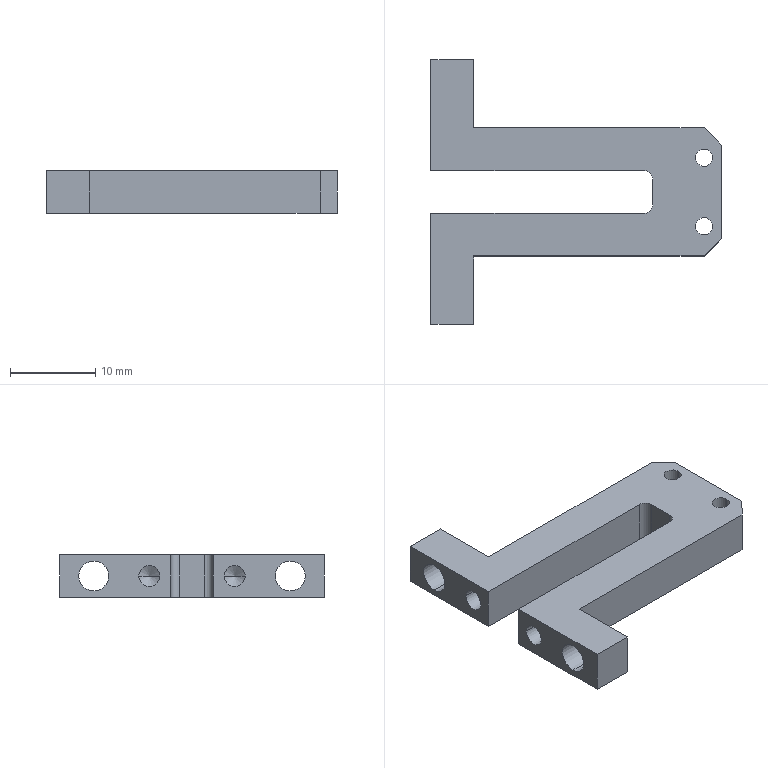Part | SolidWorks | features BaseBody 1 | 1 solid | 34 faces | box 34 x 31 x 5 mm | volume 2038 mm3 | plane 16 | cylinder 14 | cone 4 | commonest cylinder face diameters 2.013 x4 2.459 x4 3.5 x4 2 x2
STEP:
#1=CARTESIAN_POINT('',(5.454,3.851,0.));
#2=VERTEX_POINT('',#1);
#3=CARTESIAN_POINT('',(7.467,3.851,0.));
#4=VERTEX_POINT('',#3);
#5=CARTESIAN_POINT('',(6.461,3.851,0.));
#6=DIRECTION('',(0.,0.,1.));
#7=DIRECTION('',(1.,0.,0.));
#8=AXIS2_PLACEMENT_3D('',#5,#6,#7);
#9=CIRCLE('',#8,1.007);
#10=EDGE_CURVE('',#2,#4,#9,.T.);
#11=ORIENTED_EDGE('',*,*,#10,.F.);
#12=CARTESIAN_POINT('',(5.454,3.851,5.));
#13=VERTEX_POINT('',#12);
#14=CARTESIAN_POINT('',(5.454,3.851,-32.497));
#15=DIRECTION('',(0.,0.,1.));
#16=VECTOR('',#15,1000.);
#17=LINE('',#14,#16);
#18=EDGE_CURVE('',#2,#13,#17,.T.);
#19=ORIENTED_EDGE('',*,*,#18,.T.);
#20=CARTESIAN_POINT('',(7.467,3.851,5.));
#21=VERTEX_POINT('',#20);
#22=CARTESIAN_POINT('',(6.461,3.851,5.));
#23=DIRECTION('',(0.,0.,-1.));
#24=DIRECTION('',(1.,0.,0.));
#25=AXIS2_PLACEMENT_3D('',#22,#23,#24);
#26=CIRCLE('',#25,1.007);
#27=EDGE_CURVE('',#21,#13,#26,.T.);
#28=ORIENTED_EDGE('',*,*,#27,.F.);
#29=CARTESIAN_POINT('',(7.467,3.851,-32.497));
#30=DIRECTION('',(0.,0.,1.));
#31=VECTOR('',#30,1000.);
#32=LINE('',#29,#31);
#33=EDGE_CURVE('',#4,#21,#32,.T.);
#34=ORIENTED_EDGE('',*,*,#33,.F.);
#35=EDGE_LOOP('',(#11,#19,#28,#34));
#36=FACE_OUTER_BOUND('',#35,.T.);
#37=CARTESIAN_POINT('',(6.461,3.851,-32.497));
#38=DIRECTION('',(0.,0.,1.));
#39=DIRECTION('',(1.,0.,0.));
#40=AXIS2_PLACEMENT_3D('',#37,#38,#39);
#41=CYLINDRICAL_SURFACE('',#40,1.007);
#42=ADVANCED_FACE('',(#36),#41,.F.);
#43=CARTESIAN_POINT('',(5.454,-4.149,0.));
#44=VERTEX_POINT('',#43);
#45=CARTESIAN_POINT('',(7.467,-4.149,0.));
#46=VERTEX_POINT('',#45);
#47=CARTESIAN_POINT('',(6.461,-4.149,0.));
#48=DIRECTION('',(0.,0.,1.));
#49=DIRECTION('',(1.,0.,0.));
#50=AXIS2_PLACEMENT_3D('',#47,#48,#49);
#51=CIRCLE('',#50,1.007);
#52=EDGE_CURVE('',#44,#46,#51,.T.);
#53=ORIENTED_EDGE('',*,*,#52,.F.);
#54=CARTESIAN_POINT('',(5.454,-4.149,5.));
#55=VERTEX_POINT('',#54);
#56=CARTESIAN_POINT('',(5.454,-4.149,-32.497));
#57=DIRECTION('',(0.,0.,1.));
#58=VECTOR('',#57,1000.);
#59=LINE('',#56,#58);
#60=EDGE_CURVE('',#44,#55,#59,.T.);
#61=ORIENTED_EDGE('',*,*,#60,.T.);
#62=CARTESIAN_POINT('',(7.467,-4.149,5.));
#63=VERTEX_POINT('',#62);
#64=CARTESIAN_POINT('',(6.461,-4.149,5.));
#65=DIRECTION('',(0.,0.,-1.));
#66=DIRECTION('',(1.,0.,0.));
#67=AXIS2_PLACEMENT_3D('',#64,#65,#66);
#68=CIRCLE('',#67,1.007);
#69=EDGE_CURVE('',#63,#55,#68,.T.);
#70=ORIENTED_EDGE('',*,*,#69,.F.);
#71=CARTESIAN_POINT('',(7.467,-4.149,-32.497));
#72=DIRECTION('',(0.,0.,1.));
#73=VECTOR('',#72,1000.);
#74=LINE('',#71,#73);
#75=EDGE_CURVE('',#46,#63,#74,.T.);
#76=ORIENTED_EDGE('',*,*,#75,.F.);
#77=EDGE_LOOP('',(#53,#61,#70,#76));
#78=FACE_OUTER_BOUND('',#77,.T.);
#79=CARTESIAN_POINT('',(6.461,-4.149,-32.497));
#80=DIRECTION('',(0.,0.,1.));
#81=DIRECTION('',(1.,0.,0.));
#82=AXIS2_PLACEMENT_3D('',#79,#80,#81);
#83=CYLINDRICAL_SURFACE('',#82,1.007);
#84=ADVANCED_FACE('',(#78),#83,.F.);
#85=CARTESIAN_POINT('',(-13.539,6.081,2.5));
#86=VERTEX_POINT('',#85);
#87=CARTESIAN_POINT('',(-13.539,3.622,2.5));
#88=VERTEX_POINT('',#87);
#89=CARTESIAN_POINT('',(-13.539,4.851,2.5));
#90=DIRECTION('',(-1.,0.,0.));
#91=DIRECTION('',(0.,-1.,0.));
#92=AXIS2_PLACEMENT_3D('',#89,#90,#91);
#93=CIRCLE('',#92,1.23);
#94=EDGE_CURVE('',#86,#88,#93,.T.);
#95=ORIENTED_EDGE('',*,*,#94,.F.);
#96=CARTESIAN_POINT('',(-25.539,6.081,2.5));
#97=VERTEX_POINT('',#96);
#98=CARTESIAN_POINT('',(-19.539,6.081,2.5));
#99=DIRECTION('',(-1.,0.,0.));
#100=VECTOR('',#99,1000.);
#101=LINE('',#98,#100);
#102=EDGE_CURVE('',#86,#97,#101,.T.);
#103=ORIENTED_EDGE('',*,*,#102,.T.);
#104=CARTESIAN_POINT('',(-25.539,3.622,2.5));
#105=VERTEX_POINT('',#104);
#106=CARTESIAN_POINT('',(-25.539,4.851,2.5));
#107=DIRECTION('',(1.,0.,0.));
#108=DIRECTION('',(0.,-1.,0.));
#109=AXIS2_PLACEMENT_3D('',#106,#107,#108);
#110=CIRCLE('',#109,1.23);
#111=EDGE_CURVE('',#105,#97,#110,.T.);
#112=ORIENTED_EDGE('',*,*,#111,.F.);
#113=CARTESIAN_POINT('',(-19.539,3.622,2.5));
#114=DIRECTION('',(-1.,0.,0.));
#115=VECTOR('',#114,1000.);
#116=LINE('',#113,#115);
#117=EDGE_CURVE('',#88,#105,#116,.T.);
#118=ORIENTED_EDGE('',*,*,#117,.F.);
#119=EDGE_LOOP('',(#95,#103,#112,#118));
#120=FACE_OUTER_BOUND('',#119,.T.);
#121=CARTESIAN_POINT('',(-19.539,4.851,2.5));
#122=DIRECTION('',(-1.,0.,0.));
#123=DIRECTION('',(0.,-1.,0.));
#124=AXIS2_PLACEMENT_3D('',#121,#122,#123);
#125=CYLINDRICAL_SURFACE('',#124,1.23);
#126=ADVANCED_FACE('',(#120),#125,.F.);
#127=CARTESIAN_POINT('',(-25.539,11.351,4.25));
#128=VERTEX_POINT('',#127);
#129=CARTESIAN_POINT('',(-25.539,11.351,0.75));
#130=VERTEX_POINT('',#129);
#131=CARTESIAN_POINT('',(-25.539,11.351,2.5));
#132=DIRECTION('',(1.,0.,0.));
#133=DIRECTION('',(0.,0.,-1.));
#134=AXIS2_PLACEMENT_3D('',#131,#132,#133);
#135=CIRCLE('',#134,1.75);
#136=EDGE_CURVE('',#128,#130,#135,.T.);
#137=ORIENTED_EDGE('',*,*,#136,.F.);
#138=CARTESIAN_POINT('',(-20.539,11.351,4.25));
#139=VERTEX_POINT('',#138);
#140=CARTESIAN_POINT('',(-66.821,11.351,4.25));
#141=DIRECTION('',(1.,0.,0.));
#142=VECTOR('',#141,1000.);
#143=LINE('',#140,#142);
#144=EDGE_CURVE('',#128,#139,#143,.T.);
#145=ORIENTED_EDGE('',*,*,#144,.T.);
#146=CARTESIAN_POINT('',(-20.539,11.351,0.75));
#147=VERTEX_POINT('',#146);
#148=CARTESIAN_POINT('',(-20.539,11.351,2.5));
#149=DIRECTION('',(-1.,0.,0.));
#150=DIRECTION('',(0.,0.,-1.));
#151=AXIS2_PLACEMENT_3D('',#148,#149,#150);
#152=CIRCLE('',#151,1.75);
#153=EDGE_CURVE('',#147,#139,#152,.T.);
#154=ORIENTED_EDGE('',*,*,#153,.F.);
#155=CARTESIAN_POINT('',(-66.821,11.351,0.75));
#156=DIRECTION('',(1.,0.,0.));
#157=VECTOR('',#156,1000.);
#158=LINE('',#155,#157);
#159=EDGE_CURVE('',#130,#147,#158,.T.);
#160=ORIENTED_EDGE('',*,*,#159,.F.);
#161=EDGE_LOOP('',(#137,#145,#154,#160));
#162=FACE_OUTER_BOUND('',#161,.T.);
#163=CARTESIAN_POINT('',(-66.821,11.351,2.5));
#164=DIRECTION('',(1.,0.,0.));
#165=DIRECTION('',(0.,0.,-1.));
#166=AXIS2_PLACEMENT_3D('',#163,#164,#165);
#167=CYLINDRICAL_SURFACE('',#166,1.75);
#168=ADVANCED_FACE('',(#162),#167,.F.);
#169=CARTESIAN_POINT('',(-25.539,-11.649,4.25));
#170=VERTEX_POINT('',#169);
#171=CARTESIAN_POINT('',(-25.539,-11.649,0.75));
#172=VERTEX_POINT('',#171);
#173=CARTESIAN_POINT('',(-25.539,-11.649,2.5));
#174=DIRECTION('',(1.,0.,0.));
#175=DIRECTION('',(0.,0.,-1.));
#176=AXIS2_PLACEMENT_3D('',#173,#174,#175);
#177=CIRCLE('',#176,1.75);
#178=EDGE_CURVE('',#170,#172,#177,.T.);
#179=ORIENTED_EDGE('',*,*,#178,.F.);
#180=CARTESIAN_POINT('',(-20.539,-11.649,4.25));
#181=VERTEX_POINT('',#180);
#182=CARTESIAN_POINT('',(-66.821,-11.649,4.25));
#183=DIRECTION('',(1.,0.,0.));
#184=VECTOR('',#183,1000.);
#185=LINE('',#182,#184);
#186=EDGE_CURVE('',#170,#181,#185,.T.);
#187=ORIENTED_EDGE('',*,*,#186,.T.);
#188=CARTESIAN_POINT('',(-20.539,-11.649,0.75));
#189=VERTEX_POINT('',#188);
#190=CARTESIAN_POINT('',(-20.539,-11.649,2.5));
#191=DIRECTION('',(-1.,0.,0.));
#192=DIRECTION('',(0.,0.,-1.));
#193=AXIS2_PLACEMENT_3D('',#190,#191,#192);
#194=CIRCLE('',#193,1.75);
#195=EDGE_CURVE('',#189,#181,#194,.T.);
#196=ORIENTED_EDGE('',*,*,#195,.F.);
#197=CARTESIAN_POINT('',(-66.821,-11.649,0.75));
#198=DIRECTION('',(1.,0.,0.));
#199=VECTOR('',#198,1000.);
#200=LINE('',#197,#199);
#201=EDGE_CURVE('',#172,#189,#200,.T.);
#202=ORIENTED_EDGE('',*,*,#201,.F.);
#203=EDGE_LOOP('',(#179,#187,#196,#202));
#204=FACE_OUTER_BOUND('',#203,.T.);
#205=CARTESIAN_POINT('',(-66.821,-11.649,2.5));
#206=DIRECTION('',(1.,0.,0.));
#207=DIRECTION('',(0.,0.,-1.));
#208=AXIS2_PLACEMENT_3D('',#205,#206,#207);
#209=CYLINDRICAL_SURFACE('',#208,1.75);
#210=ADVANCED_FACE('',(#204),#209,.F.);
#211=CARTESIAN_POINT('',(-13.539,-3.919,2.5));
#212=VERTEX_POINT('',#211);
#213=CARTESIAN_POINT('',(-13.539,-6.378,2.5));
#214=VERTEX_POINT('',#213);
#215=CARTESIAN_POINT('',(-13.539,-5.149,2.5));
#216=DIRECTION('',(-1.,0.,0.));
#217=DIRECTION('',(0.,-1.,0.));
#218=AXIS2_PLACEMENT_3D('',#215,#216,#217);
#219=CIRCLE('',#218,1.23);
#220=EDGE_CURVE('',#212,#214,#219,.T.);
#221=ORIENTED_EDGE('',*,*,#220,.F.);
#222=CARTESIAN_POINT('',(-25.539,-3.919,2.5));
#223=VERTEX_POINT('',#222);
#224=CARTESIAN_POINT('',(-19.539,-3.919,2.5));
#225=DIRECTION('',(-1.,0.,0.));
#226=VECTOR('',#225,1000.);
#227=LINE('',#224,#226);
#228=EDGE_CURVE('',#212,#223,#227,.T.);
#229=ORIENTED_EDGE('',*,*,#228,.T.);
#230=CARTESIAN_POINT('',(-25.539,-6.378,2.5));
#231=VERTEX_POINT('',#230);
#232=CARTESIAN_POINT('',(-25.539,-5.149,2.5));
#233=DIRECTION('',(1.,0.,0.));
#234=DIRECTION('',(0.,-1.,0.));
#235=AXIS2_PLACEMENT_3D('',#232,#233,#234);
#236=CIRCLE('',#235,1.23);
#237=EDGE_CURVE('',#231,#223,#236,.T.);
#238=ORIENTED_EDGE('',*,*,#237,.F.);
#239=CARTESIAN_POINT('',(-19.539,-6.378,2.5));
#240=DIRECTION('',(-1.,0.,0.));
#241=VECTOR('',#240,1000.);
#242=LINE('',#239,#241);
#243=EDGE_CURVE('',#214,#231,#242,.T.);
#244=ORIENTED_EDGE('',*,*,#243,.F.);
#245=EDGE_LOOP('',(#221,#229,#238,#244));
#246=FACE_OUTER_BOUND('',#245,.T.);
#247=CARTESIAN_POINT('',(-19.539,-5.149,2.5));
#248=DIRECTION('',(-1.,0.,0.));
#249=DIRECTION('',(0.,-1.,0.));
#250=AXIS2_PLACEMENT_3D('',#247,#248,#249);
#251=CYLINDRICAL_SURFACE('',#250,1.23);
#252=ADVANCED_FACE('',(#246),#251,.F.);
#253=CARTESIAN_POINT('',(-12.8,4.851,2.5));
#254=VERTEX_POINT('',#253);
#255=CARTESIAN_POINT('',(-13.539,3.622,2.5));
#256=DIRECTION('',(-0.515,-0.8572,0.));
#257=VECTOR('',#256,1000.);
#258=LINE('',#255,#257);
#259=EDGE_CURVE('',#254,#88,#258,.T.);
#260=ORIENTED_EDGE('',*,*,#259,.F.);
#261=CARTESIAN_POINT('',(-13.539,6.081,2.5));
#262=DIRECTION('',(-0.515,0.8572,0.));
#263=VECTOR('',#262,1000.);
#264=LINE('',#261,#263);
#265=EDGE_CURVE('',#254,#86,#264,.T.);
#266=ORIENTED_EDGE('',*,*,#265,.T.);
#267=ORIENTED_EDGE('',*,*,#94,.T.);
#268=EDGE_LOOP('',(#260,#266,#267));
#269=FACE_OUTER_BOUND('',#268,.T.);
#270=CARTESIAN_POINT('',(-13.539,4.851,2.5));
#271=DIRECTION('',(-1.,0.,0.));
#272=DIRECTION('',(0.,-1.,0.));
#273=AXIS2_PLACEMENT_3D('',#270,#271,#272);
#274=CONICAL_SURFACE('',#273,1.229,1.03);
#275=ADVANCED_FACE('',(#269),#274,.F.);
#276=CARTESIAN_POINT('',(-12.8,-5.149,2.5));
#277=VERTEX_POINT('',#276);
#278=CARTESIAN_POINT('',(-13.539,-6.378,2.5));
#279=DIRECTION('',(-0.515,-0.8572,0.));
#280=VECTOR('',#279,1000.);
#281=LINE('',#278,#280);
#282=EDGE_CURVE('',#277,#214,#281,.T.);
#283=ORIENTED_EDGE('',*,*,#282,.F.);
#284=CARTESIAN_POINT('',(-13.539,-3.919,2.5));
#285=DIRECTION('',(-0.515,0.8572,0.));
#286=VECTOR('',#285,1000.);
#287=LINE('',#284,#286);
#288=EDGE_CURVE('',#277,#212,#287,.T.);
#289=ORIENTED_EDGE('',*,*,#288,.T.);
#290=ORIENTED_EDGE('',*,*,#220,.T.);
#291=EDGE_LOOP('',(#283,#289,#290));
#292=FACE_OUTER_BOUND('',#291,.T.);
#293=CARTESIAN_POINT('',(-13.539,-5.149,2.5));
#294=DIRECTION('',(-1.,0.,0.));
#295=DIRECTION('',(0.,-1.,0.));
#296=AXIS2_PLACEMENT_3D('',#293,#294,#295);
#297=CONICAL_SURFACE('',#296,1.229,1.03);
#298=ADVANCED_FACE('',(#292),#297,.F.);
#299=ORIENTED_EDGE('',*,*,#27,.T.);
#300=CARTESIAN_POINT('',(6.461,3.851,5.));
#301=DIRECTION('',(0.,0.,-1.));
#302=DIRECTION('',(1.,0.,0.));
#303=AXIS2_PLACEMENT_3D('',#300,#301,#302);
#304=CIRCLE('',#303,1.007);
#305=EDGE_CURVE('',#13,#21,#304,.T.);
#306=ORIENTED_EDGE('',*,*,#305,.T.);
#307=EDGE_LOOP('',(#299,#306));
#308=FACE_BOUND('',#307,.T.);
#309=ORIENTED_EDGE('',*,*,#69,.T.);
#310=CARTESIAN_POINT('',(6.461,-4.149,5.));
#311=DIRECTION('',(0.,0.,-1.));
#312=DIRECTION('',(1.,0.,0.));
#313=AXIS2_PLACEMENT_3D('',#310,#311,#312);
#314=CIRCLE('',#313,1.007);
#315=EDGE_CURVE('',#55,#63,#314,.T.);
#316=ORIENTED_EDGE('',*,*,#315,.T.);
#317=EDGE_LOOP('',(#309,#316));
#318=FACE_BOUND('',#317,.T.);
#319=CARTESIAN_POINT('',(-20.539,15.351,5.));
#320=VERTEX_POINT('',#319);
#321=CARTESIAN_POINT('',(-25.539,15.351,5.));
#322=VERTEX_POINT('',#321);
#323=CARTESIAN_POINT('',(-8.539,15.351,5.));
#324=DIRECTION('',(-1.,0.,0.));
#325=VECTOR('',#324,1000.);
#326=LINE('',#323,#325);
#327=EDGE_CURVE('',#320,#322,#326,.T.);
#328=ORIENTED_EDGE('',*,*,#327,.T.);
#329=CARTESIAN_POINT('',(-25.539,2.351,5.));
#330=VERTEX_POINT('',#329);
#331=CARTESIAN_POINT('',(-25.539,-0.1489,5.));
#332=DIRECTION('',(0.,-1.,0.));
#333=VECTOR('',#332,1000.);
#334=LINE('',#331,#333);
#335=EDGE_CURVE('',#322,#330,#334,.T.);
#336=ORIENTED_EDGE('',*,*,#335,.T.);
#337=CARTESIAN_POINT('',(-0.5392,2.351,5.));
#338=VERTEX_POINT('',#337);
#339=CARTESIAN_POINT('',(-8.539,2.351,5.));
#340=DIRECTION('',(1.,0.,0.));
#341=VECTOR('',#340,1000.);
#342=LINE('',#339,#341);
#343=EDGE_CURVE('',#330,#338,#342,.T.);
#344=ORIENTED_EDGE('',*,*,#343,.T.);
#345=CARTESIAN_POINT('',(0.4608,1.351,5.));
#346=VERTEX_POINT('',#345);
#347=CARTESIAN_POINT('',(-0.5392,1.351,5.));
#348=DIRECTION('',(0.,0.,-1.));
#349=DIRECTION('',(-1.,0.,0.));
#350=AXIS2_PLACEMENT_3D('',#347,#348,#349);
#351=CIRCLE('',#350,1.);
#352=EDGE_CURVE('',#338,#346,#351,.T.);
#353=ORIENTED_EDGE('',*,*,#352,.T.);
#354=CARTESIAN_POINT('',(0.4608,-1.649,5.));
#355=VERTEX_POINT('',#354);
#356=CARTESIAN_POINT('',(0.4608,-0.1489,5.));
#357=DIRECTION('',(0.,-1.,0.));
#358=VECTOR('',#357,1000.);
#359=LINE('',#356,#358);
#360=EDGE_CURVE('',#346,#355,#359,.T.);
#361=ORIENTED_EDGE('',*,*,#360,.T.);
#362=CARTESIAN_POINT('',(-0.5392,-2.649,5.));
#363=VERTEX_POINT('',#362);
#364=CARTESIAN_POINT('',(-0.5392,-1.649,5.));
#365=DIRECTION('',(0.,0.,-1.));
#366=DIRECTION('',(-1.,0.,0.));
#367=AXIS2_PLACEMENT_3D('',#364,#365,#366);
#368=CIRCLE('',#367,1.);
#369=EDGE_CURVE('',#355,#363,#368,.T.);
#370=ORIENTED_EDGE('',*,*,#369,.T.);
#371=CARTESIAN_POINT('',(-25.539,-2.649,5.));
#372=VERTEX_POINT('',#371);
#373=CARTESIAN_POINT('',(-8.539,-2.649,5.));
#374=DIRECTION('',(-1.,0.,0.));
#375=VECTOR('',#374,1000.);
#376=LINE('',#373,#375);
#377=EDGE_CURVE('',#363,#372,#376,.T.);
#378=ORIENTED_EDGE('',*,*,#377,.T.);
#379=CARTESIAN_POINT('',(-25.539,-15.649,5.));
#380=VERTEX_POINT('',#379);
#381=CARTESIAN_POINT('',(-25.539,-0.1489,5.));
#382=DIRECTION('',(0.,-1.,0.));
#383=VECTOR('',#382,1000.);
#384=LINE('',#381,#383);
#385=EDGE_CURVE('',#372,#380,#384,.T.);
#386=ORIENTED_EDGE('',*,*,#385,.T.);
#387=CARTESIAN_POINT('',(-20.539,-15.649,5.));
#388=VERTEX_POINT('',#387);
#389=CARTESIAN_POINT('',(-8.539,-15.649,5.));
#390=DIRECTION('',(1.,0.,0.));
#391=VECTOR('',#390,1000.);
#392=LINE('',#389,#391);
#393=EDGE_CURVE('',#380,#388,#392,.T.);
#394=ORIENTED_EDGE('',*,*,#393,.T.);
#395=CARTESIAN_POINT('',(-20.539,-7.649,5.));
#396=VERTEX_POINT('',#395);
#397=CARTESIAN_POINT('',(-20.539,-0.1489,5.));
#398=DIRECTION('',(0.,1.,0.));
#399=VECTOR('',#398,1000.);
#400=LINE('',#397,#399);
#401=EDGE_CURVE('',#388,#396,#400,.T.);
#402=ORIENTED_EDGE('',*,*,#401,.T.);
#403=CARTESIAN_POINT('',(6.461,-7.649,5.));
#404=VERTEX_POINT('',#403);
#405=CARTESIAN_POINT('',(-8.539,-7.649,5.));
#406=DIRECTION('',(1.,0.,0.));
#407=VECTOR('',#406,1000.);
#408=LINE('',#405,#407);
#409=EDGE_CURVE('',#396,#404,#408,.T.);
#410=ORIENTED_EDGE('',*,*,#409,.T.);
#411=CARTESIAN_POINT('',(8.461,-5.649,5.));
#412=VERTEX_POINT('',#411);
#413=CARTESIAN_POINT('',(6.461,-7.649,5.));
#414=DIRECTION('',(0.7071,0.7071,0.));
#415=VECTOR('',#414,1000.);
#416=LINE('',#413,#415);
#417=EDGE_CURVE('',#404,#412,#416,.T.);
#418=ORIENTED_EDGE('',*,*,#417,.T.);
#419=CARTESIAN_POINT('',(8.461,5.351,5.));
#420=VERTEX_POINT('',#419);
#421=CARTESIAN_POINT('',(8.461,-0.1489,5.));
#422=DIRECTION('',(0.,1.,0.));
#423=VECTOR('',#422,1000.);
#424=LINE('',#421,#423);
#425=EDGE_CURVE('',#412,#420,#424,.T.);
#426=ORIENTED_EDGE('',*,*,#425,.T.);
#427=CARTESIAN_POINT('',(6.461,7.351,5.));
#428=VERTEX_POINT('',#427);
#429=CARTESIAN_POINT('',(8.461,5.351,5.));
#430=DIRECTION('',(-0.7071,0.7071,0.));
#431=VECTOR('',#430,1000.);
#432=LINE('',#429,#431);
#433=EDGE_CURVE('',#420,#428,#432,.T.);
#434=ORIENTED_EDGE('',*,*,#433,.T.);
#435=CARTESIAN_POINT('',(-20.539,7.351,5.));
#436=VERTEX_POINT('',#435);
#437=CARTESIAN_POINT('',(-8.539,7.351,5.));
#438=DIRECTION('',(-1.,0.,0.));
#439=VECTOR('',#438,1000.);
#440=LINE('',#437,#439);
#441=EDGE_CURVE('',#428,#436,#440,.T.);
#442=ORIENTED_EDGE('',*,*,#441,.T.);
#443=CARTESIAN_POINT('',(-20.539,-0.1489,5.));
#444=DIRECTION('',(0.,1.,0.));
#445=VECTOR('',#444,1000.);
#446=LINE('',#443,#445);
#447=EDGE_CURVE('',#436,#320,#446,.T.);
#448=ORIENTED_EDGE('',*,*,#447,.T.);
#449=EDGE_LOOP('',(#328,#336,#344,#353,#361,#370,#378,#386,#394,#402,#410,#418,#426,#434,#442,#448));
#450=FACE_OUTER_BOUND('',#449,.T.);
#451=CARTESIAN_POINT('',(-8.539,-0.1489,5.));
#452=DIRECTION('',(0.,0.,1.));
#453=DIRECTION('',(1.,0.,0.));
#454=AXIS2_PLACEMENT_3D('',#451,#452,#453);
#455=PLANE('',#454);
#456=ADVANCED_FACE('',(#308,#318,#450),#455,.T.);
#457=ORIENTED_EDGE('',*,*,#18,.F.);
#458=CARTESIAN_POINT('',(6.461,3.851,0.));
#459=DIRECTION('',(0.,0.,1.));
#460=DIRECTION('',(1.,0.,0.));
#461=AXIS2_PLACEMENT_3D('',#458,#459,#460);
#462=CIRCLE('',#461,1.007);
#463=EDGE_CURVE('',#4,#2,#462,.T.);
#464=ORIENTED_EDGE('',*,*,#463,.F.);
#465=ORIENTED_EDGE('',*,*,#33,.T.);
#466=ORIENTED_EDGE('',*,*,#305,.F.);
#467=EDGE_LOOP('',(#457,#464,#465,#466));
#468=FACE_OUTER_BOUND('',#467,.T.);
#469=CARTESIAN_POINT('',(6.461,3.851,-32.497));
#470=DIRECTION('',(0.,0.,1.));
#471=DIRECTION('',(1.,0.,0.));
#472=AXIS2_PLACEMENT_3D('',#469,#470,#471);
#473=CYLINDRICAL_SURFACE('',#472,1.007);
#474=ADVANCED_FACE('',(#468),#473,.F.);
#475=ORIENTED_EDGE('',*,*,#60,.F.);
#476=CARTESIAN_POINT('',(6.461,-4.149,0.));
#477=DIRECTION('',(0.,0.,1.));
#478=DIRECTION('',(1.,0.,0.));
#479=AXIS2_PLACEMENT_3D('',#476,#477,#478);
#480=CIRCLE('',#479,1.007);
#481=EDGE_CURVE('',#46,#44,#480,.T.);
#482=ORIENTED_EDGE('',*,*,#481,.F.);
#483=ORIENTED_EDGE('',*,*,#75,.T.);
#484=ORIENTED_EDGE('',*,*,#315,.F.);
#485=EDGE_LOOP('',(#475,#482,#483,#484));
#486=FACE_OUTER_BOUND('',#485,.T.);
#487=CARTESIAN_POINT('',(6.461,-4.149,-32.497));
#488=DIRECTION('',(0.,0.,1.));
#489=DIRECTION('',(1.,0.,0.));
#490=AXIS2_PLACEMENT_3D('',#487,#488,#489);
#491=CYLINDRICAL_SURFACE('',#490,1.007);
#492=ADVANCED_FACE('',(#486),#491,.F.);
#493=ORIENTED_EDGE('',*,*,#111,.T.);
#494=CARTESIAN_POINT('',(-25.539,4.851,2.5));
#495=DIRECTION('',(1.,0.,0.));
#496=DIRECTION('',(0.,-1.,0.));
#497=AXIS2_PLACEMENT_3D('',#494,#495,#496);
#498=CIRCLE('',#497,1.23);
#499=EDGE_CURVE('',#97,#105,#498,.T.);
#500=ORIENTED_EDGE('',*,*,#499,.T.);
#501=EDGE_LOOP('',(#493,#500));
#502=FACE_BOUND('',#501,.T.);
#503=CARTESIAN_POINT('',(-25.539,11.351,2.5));
#504=DIRECTION('',(1.,0.,0.));
#505=DIRECTION('',(0.,0.,-1.));
#506=AXIS2_PLACEMENT_3D('',#503,#504,#505);
#507=CIRCLE('',#506,1.75);
#508=EDGE_CURVE('',#130,#128,#507,.T.);
#509=ORIENTED_EDGE('',*,*,#508,.T.);
#510=ORIENTED_EDGE('',*,*,#136,.T.);
#511=EDGE_LOOP('',(#509,#510));
#512=FACE_BOUND('',#511,.T.);
#513=CARTESIAN_POINT('',(-25.539,15.351,0.));
#514=VERTEX_POINT('',#513);
#515=CARTESIAN_POINT('',(-25.539,15.351,0.));
#516=DIRECTION('',(0.,0.,-1.));
#517=VECTOR('',#516,1000.);
#518=LINE('',#515,#517);
#519=EDGE_CURVE('',#322,#514,#518,.T.);
#520=ORIENTED_EDGE('',*,*,#519,.T.);
#521=CARTESIAN_POINT('',(-25.539,2.351,0.));
#522=VERTEX_POINT('',#521);
#523=CARTESIAN_POINT('',(-25.539,-7.649,0.));
#524=DIRECTION('',(0.,-1.,0.));
#525=VECTOR('',#524,1000.);
#526=LINE('',#523,#525);
#527=EDGE_CURVE('',#514,#522,#526,.T.);
#528=ORIENTED_EDGE('',*,*,#527,.T.);
#529=CARTESIAN_POINT('',(-25.539,2.351,0.));
#530=DIRECTION('',(0.,0.,1.));
#531=VECTOR('',#530,1000.);
#532=LINE('',#529,#531);
#533=EDGE_CURVE('',#522,#330,#532,.T.);
#534=ORIENTED_EDGE('',*,*,#533,.T.);
#535=ORIENTED_EDGE('',*,*,#335,.F.);
#536=EDGE_LOOP('',(#520,#528,#534,#535));
#537=FACE_OUTER_BOUND('',#536,.T.);
#538=CARTESIAN_POINT('',(-25.539,-7.649,0.));
#539=DIRECTION('',(-1.,0.,0.));
#540=DIRECTION('',(0.,0.,1.));
#541=AXIS2_PLACEMENT_3D('',#538,#539,#540);
#542=PLANE('',#541);
#543=ADVANCED_FACE('',(#502,#512,#537),#542,.T.);
#544=ORIENTED_EDGE('',*,*,#327,.F.);
#545=CARTESIAN_POINT('',(-20.539,15.351,0.));
#546=VERTEX_POINT('',#545);
#547=CARTESIAN_POINT('',(-20.539,15.351,2.5));
#548=DIRECTION('',(0.,0.,-1.));
#549=VECTOR('',#548,1000.);
#550=LINE('',#547,#549);
#551=EDGE_CURVE('',#320,#546,#550,.T.);
#552=ORIENTED_EDGE('',*,*,#551,.T.);
#553=CARTESIAN_POINT('',(-23.039,15.351,0.));
#554=DIRECTION('',(-1.,0.,0.));
#555=VECTOR('',#554,1000.);
#556=LINE('',#553,#555);
#557=EDGE_CURVE('',#546,#514,#556,.T.);
#558=ORIENTED_EDGE('',*,*,#557,.T.);
#559=ORIENTED_EDGE('',*,*,#519,.F.);
#560=EDGE_LOOP('',(#544,#552,#558,#559));
#561=FACE_OUTER_BOUND('',#560,.T.);
#562=CARTESIAN_POINT('',(-23.039,15.351,2.5));
#563=DIRECTION('',(0.,1.,0.));
#564=DIRECTION('',(0.,0.,1.));
#565=AXIS2_PLACEMENT_3D('',#562,#563,#564);
#566=PLANE('',#565);
#567=ADVANCED_FACE('',(#561),#566,.T.);
#568=ORIENTED_EDGE('',*,*,#153,.T.);
#569=CARTESIAN_POINT('',(-20.539,11.351,2.5));
#570=DIRECTION('',(-1.,0.,0.));
#571=DIRECTION('',(0.,0.,-1.));
#572=AXIS2_PLACEMENT_3D('',#569,#570,#571);
#573=CIRCLE('',#572,1.75);
#574=EDGE_CURVE('',#139,#147,#573,.T.);
#575=ORIENTED_EDGE('',*,*,#574,.T.);
#576=EDGE_LOOP('',(#568,#575));
#577=FACE_BOUND('',#576,.T.);
#578=CARTESIAN_POINT('',(-20.539,7.351,0.));
#579=VERTEX_POINT('',#578);
#580=CARTESIAN_POINT('',(-20.539,7.351,0.));
#581=DIRECTION('',(0.,0.,-1.));
#582=VECTOR('',#581,1000.);
#583=LINE('',#580,#582);
#584=EDGE_CURVE('',#436,#579,#583,.T.);
#585=ORIENTED_EDGE('',*,*,#584,.T.);
#586=CARTESIAN_POINT('',(-20.539,7.351,0.));
#587=DIRECTION('',(0.,1.,0.));
#588=VECTOR('',#587,1000.);
#589=LINE('',#586,#588);
#590=EDGE_CURVE('',#579,#546,#589,.T.);
#591=ORIENTED_EDGE('',*,*,#590,.T.);
#592=ORIENTED_EDGE('',*,*,#551,.F.);
#593=ORIENTED_EDGE('',*,*,#447,.F.);
#594=EDGE_LOOP('',(#585,#591,#592,#593));
#595=FACE_OUTER_BOUND('',#594,.T.);
#596=CARTESIAN_POINT('',(-20.539,7.351,0.));
#597=DIRECTION('',(1.,0.,0.));
#598=DIRECTION('',(0.,0.,-1.));
#599=AXIS2_PLACEMENT_3D('',#596,#597,#598);
#600=PLANE('',#599);
#601=ADVANCED_FACE('',(#577,#595),#600,.T.);
#602=CARTESIAN_POINT('',(6.461,7.351,0.));
#603=VERTEX_POINT('',#602);
#604=CARTESIAN_POINT('',(6.461,7.351,0.));
#605=DIRECTION('',(0.,0.,-1.));
#606=VECTOR('',#605,1000.);
#607=LINE('',#604,#606);
#608=EDGE_CURVE('',#428,#603,#607,.T.);
#609=ORIENTED_EDGE('',*,*,#608,.T.);
#610=CARTESIAN_POINT('',(-25.539,7.351,0.));
#611=DIRECTION('',(-1.,0.,0.));
#612=VECTOR('',#611,1000.);
#613=LINE('',#610,#612);
#614=EDGE_CURVE('',#603,#579,#613,.T.);
#615=ORIENTED_EDGE('',*,*,#614,.T.);
#616=ORIENTED_EDGE('',*,*,#584,.F.);
#617=ORIENTED_EDGE('',*,*,#441,.F.);
#618=EDGE_LOOP('',(#609,#615,#616,#617));
#619=FACE_OUTER_BOUND('',#618,.T.);
#620=CARTESIAN_POINT('',(-25.539,7.351,0.));
#621=DIRECTION('',(0.,1.,0.));
#622=DIRECTION('',(0.,0.,1.));
#623=AXIS2_PLACEMENT_3D('',#620,#621,#622);
#624=PLANE('',#623);
#625=ADVANCED_FACE('',(#619),#624,.T.);
#626=CARTESIAN_POINT('',(8.461,5.351,0.));
#627=VERTEX_POINT('',#626);
#628=CARTESIAN_POINT('',(7.461,6.351,0.));
#629=DIRECTION('',(-0.7071,0.7071,0.));
#630=VECTOR('',#629,1000.);
#631=LINE('',#628,#630);
#632=EDGE_CURVE('',#627,#603,#631,.T.);
#633=ORIENTED_EDGE('',*,*,#632,.T.);
#634=ORIENTED_EDGE('',*,*,#608,.F.);
#635=ORIENTED_EDGE('',*,*,#433,.F.);
#636=CARTESIAN_POINT('',(8.461,5.351,0.));
#637=DIRECTION('',(0.,0.,-1.));
#638=VECTOR('',#637,1000.);
#639=LINE('',#636,#638);
#640=EDGE_CURVE('',#420,#627,#639,.T.);
#641=ORIENTED_EDGE('',*,*,#640,.T.);
#642=EDGE_LOOP('',(#633,#634,#635,#641));
#643=FACE_OUTER_BOUND('',#642,.T.);
#644=CARTESIAN_POINT('',(7.461,6.351,0.));
#645=DIRECTION('',(0.7071,0.7071,0.));
#646=DIRECTION('',(-0.7071,0.7071,0.));
#647=AXIS2_PLACEMENT_3D('',#644,#645,#646);
#648=PLANE('',#647);
#649=ADVANCED_FACE('',(#643),#648,.T.);
#650=ORIENTED_EDGE('',*,*,#640,.F.);
#651=ORIENTED_EDGE('',*,*,#425,.F.);
#652=CARTESIAN_POINT('',(8.461,-5.649,0.));
#653=VERTEX_POINT('',#652);
#654=CARTESIAN_POINT('',(8.461,-5.649,0.));
#655=DIRECTION('',(0.,0.,-1.));
#656=VECTOR('',#655,1000.);
#657=LINE('',#654,#656);
#658=EDGE_CURVE('',#412,#653,#657,.T.);
#659=ORIENTED_EDGE('',*,*,#658,.T.);
#660=CARTESIAN_POINT('',(8.461,7.351,0.));
#661=DIRECTION('',(0.,1.,0.));
#662=VECTOR('',#661,1000.);
#663=LINE('',#660,#662);
#664=EDGE_CURVE('',#653,#627,#663,.T.);
#665=ORIENTED_EDGE('',*,*,#664,.T.);
#666=EDGE_LOOP('',(#650,#651,#659,#665));
#667=FACE_OUTER_BOUND('',#666,.T.);
#668=CARTESIAN_POINT('',(8.461,7.351,0.));
#669=DIRECTION('',(1.,0.,0.));
#670=DIRECTION('',(0.,0.,-1.));
#671=AXIS2_PLACEMENT_3D('',#668,#669,#670);
#672=PLANE('',#671);
#673=ADVANCED_FACE('',(#667),#672,.T.);
#674=CARTESIAN_POINT('',(6.461,-7.649,0.));
#675=VERTEX_POINT('',#674);
#676=CARTESIAN_POINT('',(7.461,-6.649,0.));
#677=DIRECTION('',(0.7071,0.7071,0.));
#678=VECTOR('',#677,1000.);
#679=LINE('',#676,#678);
#680=EDGE_CURVE('',#675,#653,#679,.T.);
#681=ORIENTED_EDGE('',*,*,#680,.T.);
#682=ORIENTED_EDGE('',*,*,#658,.F.);
#683=ORIENTED_EDGE('',*,*,#417,.F.);
#684=CARTESIAN_POINT('',(6.461,-7.649,0.));
#685=DIRECTION('',(0.,0.,-1.));
#686=VECTOR('',#685,1000.);
#687=LINE('',#684,#686);
#688=EDGE_CURVE('',#404,#675,#687,.T.);
#689=ORIENTED_EDGE('',*,*,#688,.T.);
#690=EDGE_LOOP('',(#681,#682,#683,#689));
#691=FACE_OUTER_BOUND('',#690,.T.);
#692=CARTESIAN_POINT('',(7.461,-6.649,0.));
#693=DIRECTION('',(0.7071,-0.7071,0.));
#694=DIRECTION('',(0.7071,0.7071,0.));
#695=AXIS2_PLACEMENT_3D('',#692,#693,#694);
#696=PLANE('',#695);
#697=ADVANCED_FACE('',(#691),#696,.T.);
#698=ORIENTED_EDGE('',*,*,#688,.F.);
#699=ORIENTED_EDGE('',*,*,#409,.F.);
#700=CARTESIAN_POINT('',(-20.539,-7.649,0.));
#701=VERTEX_POINT('',#700);
#702=CARTESIAN_POINT('',(-20.539,-7.649,0.));
#703=DIRECTION('',(0.,0.,-1.));
#704=VECTOR('',#703,1000.);
#705=LINE('',#702,#704);
#706=EDGE_CURVE('',#396,#701,#705,.T.);
#707=ORIENTED_EDGE('',*,*,#706,.T.);
#708=CARTESIAN_POINT('',(8.461,-7.649,0.));
#709=DIRECTION('',(1.,0.,0.));
#710=VECTOR('',#709,1000.);
#711=LINE('',#708,#710);
#712=EDGE_CURVE('',#701,#675,#711,.T.);
#713=ORIENTED_EDGE('',*,*,#712,.T.);
#714=EDGE_LOOP('',(#698,#699,#707,#713));
#715=FACE_OUTER_BOUND('',#714,.T.);
#716=CARTESIAN_POINT('',(8.461,-7.649,0.));
#717=DIRECTION('',(0.,-1.,0.));
#718=DIRECTION('',(0.,0.,-1.));
#719=AXIS2_PLACEMENT_3D('',#716,#717,#718);
#720=PLANE('',#719);
#721=ADVANCED_FACE('',(#715),#720,.T.);
#722=ORIENTED_EDGE('',*,*,#195,.T.);
#723=CARTESIAN_POINT('',(-20.539,-11.649,2.5));
#724=DIRECTION('',(-1.,0.,0.));
#725=DIRECTION('',(0.,0.,-1.));
#726=AXIS2_PLACEMENT_3D('',#723,#724,#725);
#727=CIRCLE('',#726,1.75);
#728=EDGE_CURVE('',#181,#189,#727,.T.);
#729=ORIENTED_EDGE('',*,*,#728,.T.);
#730=EDGE_LOOP('',(#722,#729));
#731=FACE_BOUND('',#730,.T.);
#732=ORIENTED_EDGE('',*,*,#706,.F.);
#733=ORIENTED_EDGE('',*,*,#401,.F.);
#734=CARTESIAN_POINT('',(-20.539,-15.649,0.));
#735=VERTEX_POINT('',#734);
#736=CARTESIAN_POINT('',(-20.539,-15.649,5.));
#737=DIRECTION('',(0.,0.,-1.));
#738=VECTOR('',#737,1000.);
#739=LINE('',#736,#738);
#740=EDGE_CURVE('',#388,#735,#739,.T.);
#741=ORIENTED_EDGE('',*,*,#740,.T.);
#742=CARTESIAN_POINT('',(-20.539,-7.649,0.));
#743=DIRECTION('',(0.,1.,0.));
#744=VECTOR('',#743,1000.);
#745=LINE('',#742,#744);
#746=EDGE_CURVE('',#735,#701,#745,.T.);
#747=ORIENTED_EDGE('',*,*,#746,.T.);
#748=EDGE_LOOP('',(#732,#733,#741,#747));
#749=FACE_OUTER_BOUND('',#748,.T.);
#750=CARTESIAN_POINT('',(-20.539,-7.649,5.));
#751=DIRECTION('',(1.,0.,0.));
#752=DIRECTION('',(0.,0.,-1.));
#753=AXIS2_PLACEMENT_3D('',#750,#751,#752);
#754=PLANE('',#753);
#755=ADVANCED_FACE('',(#731,#749),#754,.T.);
#756=CARTESIAN_POINT('',(-25.539,-15.649,0.));
#757=VERTEX_POINT('',#756);
#758=CARTESIAN_POINT('',(-25.539,-15.649,2.5));
#759=DIRECTION('',(0.,0.,1.));
#760=VECTOR('',#759,1000.);
#761=LINE('',#758,#760);
#762=EDGE_CURVE('',#757,#380,#761,.T.);
#763=ORIENTED_EDGE('',*,*,#762,.F.);
#764=CARTESIAN_POINT('',(-23.039,-15.649,0.));
#765=DIRECTION('',(-1.,0.,0.));
#766=VECTOR('',#765,1000.);
#767=LINE('',#764,#766);
#768=EDGE_CURVE('',#735,#757,#767,.T.);
#769=ORIENTED_EDGE('',*,*,#768,.F.);
#770=ORIENTED_EDGE('',*,*,#740,.F.);
#771=ORIENTED_EDGE('',*,*,#393,.F.);
#772=EDGE_LOOP('',(#763,#769,#770,#771));
#773=FACE_OUTER_BOUND('',#772,.T.);
#774=CARTESIAN_POINT('',(-23.039,-15.649,2.5));
#775=DIRECTION('',(0.,1.,0.));
#776=DIRECTION('',(0.,0.,1.));
#777=AXIS2_PLACEMENT_3D('',#774,#775,#776);
#778=PLANE('',#777);
#779=ADVANCED_FACE('',(#773),#778,.F.);
#780=ORIENTED_EDGE('',*,*,#237,.T.);
#781=CARTESIAN_POINT('',(-25.539,-5.149,2.5));
#782=DIRECTION('',(1.,0.,0.));
#783=DIRECTION('',(0.,-1.,0.));
#784=AXIS2_PLACEMENT_3D('',#781,#782,#783);
#785=CIRCLE('',#784,1.23);
#786=EDGE_CURVE('',#223,#231,#785,.T.);
#787=ORIENTED_EDGE('',*,*,#786,.T.);
#788=EDGE_LOOP('',(#780,#787));
#789=FACE_BOUND('',#788,.T.);
#790=CARTESIAN_POINT('',(-25.539,-11.649,2.5));
#791=DIRECTION('',(1.,0.,0.));
#792=DIRECTION('',(0.,0.,-1.));
#793=AXIS2_PLACEMENT_3D('',#790,#791,#792);
#794=CIRCLE('',#793,1.75);
#795=EDGE_CURVE('',#172,#170,#794,.T.);
#796=ORIENTED_EDGE('',*,*,#795,.T.);
#797=ORIENTED_EDGE('',*,*,#178,.T.);
#798=EDGE_LOOP('',(#796,#797));
#799=FACE_BOUND('',#798,.T.);
#800=ORIENTED_EDGE('',*,*,#762,.T.);
#801=ORIENTED_EDGE('',*,*,#385,.F.);
#802=CARTESIAN_POINT('',(-25.539,-2.649,0.));
#803=VERTEX_POINT('',#802);
#804=CARTESIAN_POINT('',(-25.539,-2.649,0.));
#805=DIRECTION('',(0.,0.,-1.));
#806=VECTOR('',#805,1000.);
#807=LINE('',#804,#806);
#808=EDGE_CURVE('',#372,#803,#807,.T.);
#809=ORIENTED_EDGE('',*,*,#808,.T.);
#810=CARTESIAN_POINT('',(-25.539,-7.649,0.));
#811=DIRECTION('',(0.,-1.,0.));
#812=VECTOR('',#811,1000.);
#813=LINE('',#810,#812);
#814=EDGE_CURVE('',#803,#757,#813,.T.);
#815=ORIENTED_EDGE('',*,*,#814,.T.);
#816=EDGE_LOOP('',(#800,#801,#809,#815));
#817=FACE_OUTER_BOUND('',#816,.T.);
#818=CARTESIAN_POINT('',(-25.539,-7.649,0.));
#819=DIRECTION('',(-1.,0.,0.));
#820=DIRECTION('',(0.,0.,1.));
#821=AXIS2_PLACEMENT_3D('',#818,#819,#820);
#822=PLANE('',#821);
#823=ADVANCED_FACE('',(#789,#799,#817),#822,.T.);
#824=CARTESIAN_POINT('',(-0.5392,-2.649,0.));
#825=VERTEX_POINT('',#824);
#826=CARTESIAN_POINT('',(-25.539,-2.649,0.));
#827=DIRECTION('',(1.,0.,0.));
#828=VECTOR('',#827,1000.);
#829=LINE('',#826,#828);
#830=EDGE_CURVE('',#803,#825,#829,.T.);
#831=ORIENTED_EDGE('',*,*,#830,.F.);
#832=ORIENTED_EDGE('',*,*,#808,.F.);
#833=ORIENTED_EDGE('',*,*,#377,.F.);
#834=CARTESIAN_POINT('',(-0.5392,-2.649,5.));
#835=DIRECTION('',(0.,0.,1.));
#836=VECTOR('',#835,1000.);
#837=LINE('',#834,#836);
#838=EDGE_CURVE('',#825,#363,#837,.T.);
#839=ORIENTED_EDGE('',*,*,#838,.F.);
#840=EDGE_LOOP('',(#831,#832,#833,#839));
#841=FACE_OUTER_BOUND('',#840,.T.);
#842=CARTESIAN_POINT('',(-25.539,-2.649,5.));
#843=DIRECTION('',(0.,-1.,0.));
#844=DIRECTION('',(0.,0.,-1.));
#845=AXIS2_PLACEMENT_3D('',#842,#843,#844);
#846=PLANE('',#845);
#847=ADVANCED_FACE('',(#841),#846,.F.);
#848=ORIENTED_EDGE('',*,*,#360,.F.);
#849=CARTESIAN_POINT('',(0.4608,1.351,0.));
#850=VERTEX_POINT('',#849);
#851=CARTESIAN_POINT('',(0.4608,1.351,5.));
#852=DIRECTION('',(0.,0.,1.));
#853=VECTOR('',#852,1000.);
#854=LINE('',#851,#853);
#855=EDGE_CURVE('',#850,#346,#854,.T.);
#856=ORIENTED_EDGE('',*,*,#855,.F.);
#857=CARTESIAN_POINT('',(0.4608,-1.649,0.));
#858=VERTEX_POINT('',#857);
#859=CARTESIAN_POINT('',(0.4608,-2.649,0.));
#860=DIRECTION('',(0.,1.,0.));
#861=VECTOR('',#860,1000.);
#862=LINE('',#859,#861);
#863=EDGE_CURVE('',#858,#850,#862,.T.);
#864=ORIENTED_EDGE('',*,*,#863,.F.);
#865=CARTESIAN_POINT('',(0.4608,-1.649,5.));
#866=DIRECTION('',(0.,0.,-1.));
#867=VECTOR('',#866,1000.);
#868=LINE('',#865,#867);
#869=EDGE_CURVE('',#355,#858,#868,.T.);
#870=ORIENTED_EDGE('',*,*,#869,.F.);
#871=EDGE_LOOP('',(#848,#856,#864,#870));
#872=FACE_OUTER_BOUND('',#871,.T.);
#873=CARTESIAN_POINT('',(0.4608,-2.649,5.));
#874=DIRECTION('',(1.,0.,0.));
#875=DIRECTION('',(0.,0.,-1.));
#876=AXIS2_PLACEMENT_3D('',#873,#874,#875);
#877=PLANE('',#876);
#878=ADVANCED_FACE('',(#872),#877,.F.);
#879=ORIENTED_EDGE('',*,*,#343,.F.);
#880=ORIENTED_EDGE('',*,*,#533,.F.);
#881=CARTESIAN_POINT('',(-0.5392,2.351,0.));
#882=VERTEX_POINT('',#881);
#883=CARTESIAN_POINT('',(0.4608,2.351,0.));
#884=DIRECTION('',(-1.,0.,0.));
#885=VECTOR('',#884,1000.);
#886=LINE('',#883,#885);
#887=EDGE_CURVE('',#882,#522,#886,.T.);
#888=ORIENTED_EDGE('',*,*,#887,.F.);
#889=CARTESIAN_POINT('',(-0.5392,2.351,5.));
#890=DIRECTION('',(0.,0.,-1.));
#891=VECTOR('',#890,1000.);
#892=LINE('',#889,#891);
#893=EDGE_CURVE('',#338,#882,#892,.T.);
#894=ORIENTED_EDGE('',*,*,#893,.F.);
#895=EDGE_LOOP('',(#879,#880,#888,#894));
#896=FACE_OUTER_BOUND('',#895,.T.);
#897=CARTESIAN_POINT('',(0.4608,2.351,5.));
#898=DIRECTION('',(0.,1.,0.));
#899=DIRECTION('',(0.,0.,1.));
#900=AXIS2_PLACEMENT_3D('',#897,#898,#899);
#901=PLANE('',#900);
#902=ADVANCED_FACE('',(#896),#901,.F.);
#903=ORIENTED_EDGE('',*,*,#463,.T.);
#904=ORIENTED_EDGE('',*,*,#10,.T.);
#905=EDGE_LOOP('',(#903,#904));
#906=FACE_BOUND('',#905,.T.);
#907=ORIENTED_EDGE('',*,*,#481,.T.);
#908=ORIENTED_EDGE('',*,*,#52,.T.);
#909=EDGE_LOOP('',(#907,#908));
#910=FACE_BOUND('',#909,.T.);
#911=ORIENTED_EDGE('',*,*,#527,.F.);
#912=ORIENTED_EDGE('',*,*,#557,.F.);
#913=ORIENTED_EDGE('',*,*,#590,.F.);
#914=ORIENTED_EDGE('',*,*,#614,.F.);
#915=ORIENTED_EDGE('',*,*,#632,.F.);
#916=ORIENTED_EDGE('',*,*,#664,.F.);
#917=ORIENTED_EDGE('',*,*,#680,.F.);
#918=ORIENTED_EDGE('',*,*,#712,.F.);
#919=ORIENTED_EDGE('',*,*,#746,.F.);
#920=ORIENTED_EDGE('',*,*,#768,.T.);
#921=ORIENTED_EDGE('',*,*,#814,.F.);
#922=ORIENTED_EDGE('',*,*,#830,.T.);
#923=CARTESIAN_POINT('',(-0.5392,-1.649,0.));
#924=DIRECTION('',(0.,0.,-1.));
#925=DIRECTION('',(-1.,0.,0.));
#926=AXIS2_PLACEMENT_3D('',#923,#924,#925);
#927=CIRCLE('',#926,1.);
#928=EDGE_CURVE('',#858,#825,#927,.T.);
#929=ORIENTED_EDGE('',*,*,#928,.F.);
#930=ORIENTED_EDGE('',*,*,#863,.T.);
#931=CARTESIAN_POINT('',(-0.5392,1.351,0.));
#932=DIRECTION('',(0.,0.,-1.));
#933=DIRECTION('',(-1.,0.,0.));
#934=AXIS2_PLACEMENT_3D('',#931,#932,#933);
#935=CIRCLE('',#934,1.);
#936=EDGE_CURVE('',#882,#850,#935,.T.);
#937=ORIENTED_EDGE('',*,*,#936,.F.);
#938=ORIENTED_EDGE('',*,*,#887,.T.);
#939=EDGE_LOOP('',(#911,#912,#913,#914,#915,#916,#917,#918,#919,#920,#921,#922,#929,#930,#937,#938));
#940=FACE_OUTER_BOUND('',#939,.T.);
#941=CARTESIAN_POINT('',(-8.539,-0.1489,0.));
#942=DIRECTION('',(0.,0.,1.));
#943=DIRECTION('',(1.,0.,0.));
#944=AXIS2_PLACEMENT_3D('',#941,#942,#943);
#945=PLANE('',#944);
#946=ADVANCED_FACE('',(#906,#910,#940),#945,.F.);
#947=ORIENTED_EDGE('',*,*,#102,.F.);
#948=CARTESIAN_POINT('',(-13.539,4.851,2.5));
#949=DIRECTION('',(-1.,0.,0.));
#950=DIRECTION('',(0.,-1.,0.));
#951=AXIS2_PLACEMENT_3D('',#948,#949,#950);
#952=CIRCLE('',#951,1.23);
#953=EDGE_CURVE('',#88,#86,#952,.T.);
#954=ORIENTED_EDGE('',*,*,#953,.F.);
#955=ORIENTED_EDGE('',*,*,#117,.T.);
#956=ORIENTED_EDGE('',*,*,#499,.F.);
#957=EDGE_LOOP('',(#947,#954,#955,#956));
#958=FACE_OUTER_BOUND('',#957,.T.);
#959=CARTESIAN_POINT('',(-19.539,4.851,2.5));
#960=DIRECTION('',(-1.,0.,0.));
#961=DIRECTION('',(0.,-1.,0.));
#962=AXIS2_PLACEMENT_3D('',#959,#960,#961);
#963=CYLINDRICAL_SURFACE('',#962,1.23);
#964=ADVANCED_FACE('',(#958),#963,.F.);
#965=ORIENTED_EDGE('',*,*,#144,.F.);
#966=ORIENTED_EDGE('',*,*,#508,.F.);
#967=ORIENTED_EDGE('',*,*,#159,.T.);
#968=ORIENTED_EDGE('',*,*,#574,.F.);
#969=EDGE_LOOP('',(#965,#966,#967,#968));
#970=FACE_OUTER_BOUND('',#969,.T.);
#971=CARTESIAN_POINT('',(-66.821,11.351,2.5));
#972=DIRECTION('',(1.,0.,0.));
#973=DIRECTION('',(0.,0.,-1.));
#974=AXIS2_PLACEMENT_3D('',#971,#972,#973);
#975=CYLINDRICAL_SURFACE('',#974,1.75);
#976=ADVANCED_FACE('',(#970),#975,.F.);
#977=ORIENTED_EDGE('',*,*,#186,.F.);
#978=ORIENTED_EDGE('',*,*,#795,.F.);
#979=ORIENTED_EDGE('',*,*,#201,.T.);
#980=ORIENTED_EDGE('',*,*,#728,.F.);
#981=EDGE_LOOP('',(#977,#978,#979,#980));
#982=FACE_OUTER_BOUND('',#981,.T.);
#983=CARTESIAN_POINT('',(-66.821,-11.649,2.5));
#984=DIRECTION('',(1.,0.,0.));
#985=DIRECTION('',(0.,0.,-1.));
#986=AXIS2_PLACEMENT_3D('',#983,#984,#985);
#987=CYLINDRICAL_SURFACE('',#986,1.75);
#988=ADVANCED_FACE('',(#982),#987,.F.);
#989=ORIENTED_EDGE('',*,*,#228,.F.);
#990=CARTESIAN_POINT('',(-13.539,-5.149,2.5));
#991=DIRECTION('',(-1.,0.,0.));
#992=DIRECTION('',(0.,-1.,0.));
#993=AXIS2_PLACEMENT_3D('',#990,#991,#992);
#994=CIRCLE('',#993,1.23);
#995=EDGE_CURVE('',#214,#212,#994,.T.);
#996=ORIENTED_EDGE('',*,*,#995,.F.);
#997=ORIENTED_EDGE('',*,*,#243,.T.);
#998=ORIENTED_EDGE('',*,*,#786,.F.);
#999=EDGE_LOOP('',(#989,#996,#997,#998));
#1000=FACE_OUTER_BOUND('',#999,.T.);
#1001=CARTESIAN_POINT('',(-19.539,-5.149,2.5));
#1002=DIRECTION('',(-1.,0.,0.));
#1003=DIRECTION('',(0.,-1.,0.));
#1004=AXIS2_PLACEMENT_3D('',#1001,#1002,#1003);
#1005=CYLINDRICAL_SURFACE('',#1004,1.23);
#1006=ADVANCED_FACE('',(#1000),#1005,.F.);
#1007=ORIENTED_EDGE('',*,*,#869,.T.);
#1008=ORIENTED_EDGE('',*,*,#928,.T.);
#1009=ORIENTED_EDGE('',*,*,#838,.T.);
#1010=ORIENTED_EDGE('',*,*,#369,.F.);
#1011=EDGE_LOOP('',(#1007,#1008,#1009,#1010));
#1012=FACE_OUTER_BOUND('',#1011,.T.);
#1013=CARTESIAN_POINT('',(-0.5392,-1.649,5.));
#1014=DIRECTION('',(0.,0.,-1.));
#1015=DIRECTION('',(-1.,0.,0.));
#1016=AXIS2_PLACEMENT_3D('',#1013,#1014,#1015);
#1017=CYLINDRICAL_SURFACE('',#1016,1.);
#1018=ADVANCED_FACE('',(#1012),#1017,.F.);
#1019=ORIENTED_EDGE('',*,*,#893,.T.);
#1020=ORIENTED_EDGE('',*,*,#936,.T.);
#1021=ORIENTED_EDGE('',*,*,#855,.T.);
#1022=ORIENTED_EDGE('',*,*,#352,.F.);
#1023=EDGE_LOOP('',(#1019,#1020,#1021,#1022));
#1024=FACE_OUTER_BOUND('',#1023,.T.);
#1025=CARTESIAN_POINT('',(-0.5392,1.351,5.));
#1026=DIRECTION('',(0.,0.,-1.));
#1027=DIRECTION('',(-1.,0.,0.));
#1028=AXIS2_PLACEMENT_3D('',#1025,#1026,#1027);
#1029=CYLINDRICAL_SURFACE('',#1028,1.);
#1030=ADVANCED_FACE('',(#1024),#1029,.F.);
#1031=ORIENTED_EDGE('',*,*,#265,.F.);
#1032=ORIENTED_EDGE('',*,*,#259,.T.);
#1033=ORIENTED_EDGE('',*,*,#953,.T.);
#1034=EDGE_LOOP('',(#1031,#1032,#1033));
#1035=FACE_OUTER_BOUND('',#1034,.T.);
#1036=CARTESIAN_POINT('',(-13.539,4.851,2.5));
#1037=DIRECTION('',(-1.,0.,0.));
#1038=DIRECTION('',(0.,-1.,0.));
#1039=AXIS2_PLACEMENT_3D('',#1036,#1037,#1038);
#1040=CONICAL_SURFACE('',#1039,1.229,1.03);
#1041=ADVANCED_FACE('',(#1035),#1040,.F.);
#1042=ORIENTED_EDGE('',*,*,#288,.F.);
#1043=ORIENTED_EDGE('',*,*,#282,.T.);
#1044=ORIENTED_EDGE('',*,*,#995,.T.);
#1045=EDGE_LOOP('',(#1042,#1043,#1044));
#1046=FACE_OUTER_BOUND('',#1045,.T.);
#1047=CARTESIAN_POINT('',(-13.539,-5.149,2.5));
#1048=DIRECTION('',(-1.,0.,0.));
#1049=DIRECTION('',(0.,-1.,0.));
#1050=AXIS2_PLACEMENT_3D('',#1047,#1048,#1049);
#1051=CONICAL_SURFACE('',#1050,1.229,1.03);
#1052=ADVANCED_FACE('',(#1046),#1051,.F.);
#1053=CLOSED_SHELL('',(#42,#84,#126,#168,#210,#252,#275,#298,#456,#474,#492,#543,#567,#601,#625,#649,#673,#697,#721,#755,#779,#823,#847,#878,#902,#946,#964,#976,#988,#1006,#1018,#1030,#1041,#1052));
#1054=MANIFOLD_SOLID_BREP('',#1053);
#1055=CARTESIAN_POINT('',(0.,0.,0.));
#1056=DIRECTION('',(0.,0.,1.));
#1057=DIRECTION('',(1.,0.,0.));
#1058=AXIS2_PLACEMENT_3D('',#1055,#1056,#1057);
#1059=(LENGTH_UNIT()NAMED_UNIT(*)SI_UNIT(.MILLI.,.METRE.));
#1060=UNCERTAINTY_MEASURE_WITH_UNIT(LENGTH_MEASURE(0.00001),#1059,'','');
#1061=(NAMED_UNIT(*)PLANE_ANGLE_UNIT()SI_UNIT($,.RADIAN.));
#1062=(NAMED_UNIT(*)SI_UNIT($,.STERADIAN.)SOLID_ANGLE_UNIT());
#1063=(GEOMETRIC_REPRESENTATION_CONTEXT(3)GLOBAL_UNCERTAINTY_ASSIGNED_CONTEXT((#1060))GLOBAL_UNIT_ASSIGNED_CONTEXT((#1059,#1061,#1062))REPRESENTATION_CONTEXT('',''));
#1064=ADVANCED_BREP_SHAPE_REPRESENTATION('',(#1054,#1058),#1063);